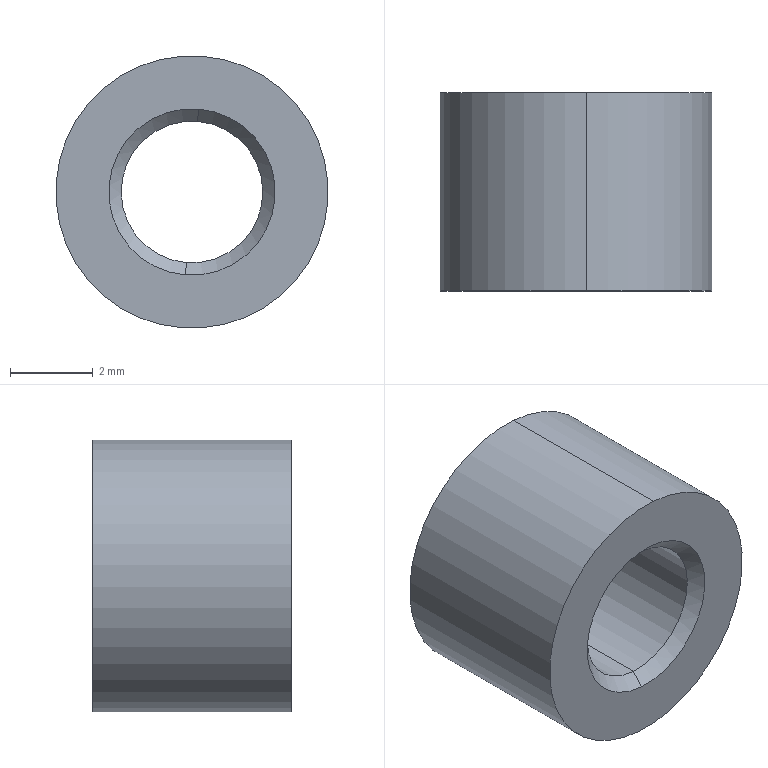Part | STEP file | 2026.6.15-Main Assembly图.sldasm-Part-262 | 1 solid | 10 faces | box 6.6 x 4.8 x 6.6 mm | volume 118.747 mm3 | cylinder 4 | cone 4 | plane 2 | commonest cylinder face diameters 3.433 x2 6.6 x2
STEP:
#1=CARTESIAN_POINT('',(-1616.254,1435.064,3409.798));
#2=VERTEX_POINT('',#1);
#3=CARTESIAN_POINT('',(-1616.254,1439.264,3409.798));
#4=VERTEX_POINT('',#3);
#5=CARTESIAN_POINT('',(-1616.254,1439.564,3409.798));
#6=DIRECTION('',(0.,1.,0.));
#7=VECTOR('',#6,1000.);
#8=LINE('',#5,#7);
#9=EDGE_CURVE('',#2,#4,#8,.T.);
#10=ORIENTED_EDGE('',*,*,#9,.F.);
#11=CARTESIAN_POINT('',(-1616.523,1435.064,3406.375));
#12=VERTEX_POINT('',#11);
#13=CARTESIAN_POINT('',(-1616.388,1435.064,3408.086));
#14=DIRECTION('',(0.,-1.,0.));
#15=DIRECTION('',(0.0785,0.,0.9969));
#16=AXIS2_PLACEMENT_3D('',#13,#14,#15);
#17=CIRCLE('',#16,1.717);
#18=EDGE_CURVE('',#2,#12,#17,.T.);
#19=ORIENTED_EDGE('',*,*,#18,.T.);
#20=CARTESIAN_POINT('',(-1616.523,1439.264,3406.375));
#21=VERTEX_POINT('',#20);
#22=CARTESIAN_POINT('',(-1616.523,1439.564,3406.375));
#23=DIRECTION('',(0.,1.,0.));
#24=VECTOR('',#23,1000.);
#25=LINE('',#22,#24);
#26=EDGE_CURVE('',#12,#21,#25,.T.);
#27=ORIENTED_EDGE('',*,*,#26,.T.);
#28=CARTESIAN_POINT('',(-1616.388,1439.264,3408.086));
#29=DIRECTION('',(0.,1.,0.));
#30=DIRECTION('',(-0.0785,0.,-0.9969));
#31=AXIS2_PLACEMENT_3D('',#28,#29,#30);
#32=CIRCLE('',#31,1.717);
#33=EDGE_CURVE('',#21,#4,#32,.T.);
#34=ORIENTED_EDGE('',*,*,#33,.T.);
#35=EDGE_LOOP('',(#10,#19,#27,#34));
#36=FACE_OUTER_BOUND('',#35,.T.);
#37=CARTESIAN_POINT('',(-1616.388,1439.564,3408.086));
#38=DIRECTION('',(0.,1.,0.));
#39=DIRECTION('',(0.0785,0.,0.9969));
#40=AXIS2_PLACEMENT_3D('',#37,#38,#39);
#41=CYLINDRICAL_SURFACE('',#40,1.717);
#42=ADVANCED_FACE('',(#36),#41,.F.);
#43=CARTESIAN_POINT('',(-1616.547,1434.764,3406.076));
#44=VERTEX_POINT('',#43);
#45=CARTESIAN_POINT('',(-1616.547,1434.764,3406.076));
#46=DIRECTION('',(0.0555,0.7071,0.7049));
#47=VECTOR('',#46,1000.);
#48=LINE('',#45,#47);
#49=EDGE_CURVE('',#44,#12,#48,.T.);
#50=ORIENTED_EDGE('',*,*,#49,.T.);
#51=ORIENTED_EDGE('',*,*,#18,.F.);
#52=CARTESIAN_POINT('',(-1616.23,1434.764,3410.097));
#53=VERTEX_POINT('',#52);
#54=CARTESIAN_POINT('',(-1616.23,1434.764,3410.097));
#55=DIRECTION('',(-0.0555,0.7071,-0.7049));
#56=VECTOR('',#55,1000.);
#57=LINE('',#54,#56);
#58=EDGE_CURVE('',#53,#2,#57,.T.);
#59=ORIENTED_EDGE('',*,*,#58,.F.);
#60=CARTESIAN_POINT('',(-1616.388,1434.764,3408.086));
#61=DIRECTION('',(0.,1.,0.));
#62=DIRECTION('',(0.0785,0.,0.9969));
#63=AXIS2_PLACEMENT_3D('',#60,#61,#62);
#64=CIRCLE('',#63,2.017);
#65=EDGE_CURVE('',#44,#53,#64,.T.);
#66=ORIENTED_EDGE('',*,*,#65,.F.);
#67=EDGE_LOOP('',(#50,#51,#59,#66));
#68=FACE_OUTER_BOUND('',#67,.T.);
#69=CARTESIAN_POINT('',(-1616.388,1434.764,3408.086));
#70=DIRECTION('',(0.,-1.,0.));
#71=DIRECTION('',(-0.0785,0.,-0.9969));
#72=AXIS2_PLACEMENT_3D('',#69,#70,#71);
#73=CONICAL_SURFACE('',#72,2.017,0.7854);
#74=ADVANCED_FACE('',(#68),#73,.F.);
#75=CARTESIAN_POINT('',(-1616.23,1439.564,3410.097));
#76=VERTEX_POINT('',#75);
#77=CARTESIAN_POINT('',(-1616.23,1439.564,3410.097));
#78=DIRECTION('',(0.0555,0.7071,0.7049));
#79=VECTOR('',#78,1000.);
#80=LINE('',#77,#79);
#81=EDGE_CURVE('',#4,#76,#80,.T.);
#82=ORIENTED_EDGE('',*,*,#81,.F.);
#83=ORIENTED_EDGE('',*,*,#33,.F.);
#84=CARTESIAN_POINT('',(-1616.547,1439.564,3406.076));
#85=VERTEX_POINT('',#84);
#86=CARTESIAN_POINT('',(-1616.547,1439.564,3406.076));
#87=DIRECTION('',(-0.0555,0.7071,-0.7049));
#88=VECTOR('',#87,1000.);
#89=LINE('',#86,#88);
#90=EDGE_CURVE('',#21,#85,#89,.T.);
#91=ORIENTED_EDGE('',*,*,#90,.T.);
#92=CARTESIAN_POINT('',(-1616.388,1439.564,3408.086));
#93=DIRECTION('',(0.,1.,0.));
#94=DIRECTION('',(-0.0785,0.,-0.9969));
#95=AXIS2_PLACEMENT_3D('',#92,#93,#94);
#96=CIRCLE('',#95,2.017);
#97=EDGE_CURVE('',#85,#76,#96,.T.);
#98=ORIENTED_EDGE('',*,*,#97,.T.);
#99=EDGE_LOOP('',(#82,#83,#91,#98));
#100=FACE_OUTER_BOUND('',#99,.T.);
#101=CARTESIAN_POINT('',(-1616.388,1439.564,3408.086));
#102=DIRECTION('',(0.,1.,0.));
#103=DIRECTION('',(0.0785,0.,0.9969));
#104=AXIS2_PLACEMENT_3D('',#101,#102,#103);
#105=CONICAL_SURFACE('',#104,2.017,0.7854);
#106=ADVANCED_FACE('',(#100),#105,.F.);
#107=CARTESIAN_POINT('',(-1616.647,1434.764,3404.797));
#108=VERTEX_POINT('',#107);
#109=CARTESIAN_POINT('',(-1616.129,1434.764,3411.376));
#110=VERTEX_POINT('',#109);
#111=CARTESIAN_POINT('',(-1616.388,1434.764,3408.086));
#112=DIRECTION('',(0.,1.,0.));
#113=DIRECTION('',(-0.0785,0.,-0.9969));
#114=AXIS2_PLACEMENT_3D('',#111,#112,#113);
#115=CIRCLE('',#114,3.3);
#116=EDGE_CURVE('',#108,#110,#115,.T.);
#117=ORIENTED_EDGE('',*,*,#116,.F.);
#118=CARTESIAN_POINT('',(-1616.388,1434.764,3408.086));
#119=DIRECTION('',(0.,1.,0.));
#120=DIRECTION('',(-0.0785,0.,-0.9969));
#121=AXIS2_PLACEMENT_3D('',#118,#119,#120);
#122=CIRCLE('',#121,3.3);
#123=EDGE_CURVE('',#110,#108,#122,.T.);
#124=ORIENTED_EDGE('',*,*,#123,.F.);
#125=EDGE_LOOP('',(#117,#124));
#126=FACE_OUTER_BOUND('',#125,.T.);
#127=CARTESIAN_POINT('',(-1616.388,1434.764,3408.086));
#128=DIRECTION('',(0.,1.,0.));
#129=DIRECTION('',(0.0785,0.,0.9969));
#130=AXIS2_PLACEMENT_3D('',#127,#128,#129);
#131=CIRCLE('',#130,2.017);
#132=EDGE_CURVE('',#53,#44,#131,.T.);
#133=ORIENTED_EDGE('',*,*,#132,.T.);
#134=ORIENTED_EDGE('',*,*,#65,.T.);
#135=EDGE_LOOP('',(#133,#134));
#136=FACE_BOUND('',#135,.T.);
#137=CARTESIAN_POINT('',(-1616.388,1434.764,3408.086));
#138=DIRECTION('',(0.,-1.,0.));
#139=DIRECTION('',(0.,0.,-1.));
#140=AXIS2_PLACEMENT_3D('',#137,#138,#139);
#141=PLANE('',#140);
#142=ADVANCED_FACE('',(#126,#136),#141,.T.);
#143=CARTESIAN_POINT('',(-1616.647,1439.564,3404.797));
#144=VERTEX_POINT('',#143);
#145=CARTESIAN_POINT('',(-1616.129,1439.564,3411.376));
#146=VERTEX_POINT('',#145);
#147=CARTESIAN_POINT('',(-1616.388,1439.564,3408.086));
#148=DIRECTION('',(0.,-1.,0.));
#149=DIRECTION('',(-0.0785,0.,-0.9969));
#150=AXIS2_PLACEMENT_3D('',#147,#148,#149);
#151=CIRCLE('',#150,3.3);
#152=EDGE_CURVE('',#144,#146,#151,.T.);
#153=ORIENTED_EDGE('',*,*,#152,.F.);
#154=CARTESIAN_POINT('',(-1616.388,1439.564,3408.086));
#155=DIRECTION('',(0.,-1.,0.));
#156=DIRECTION('',(-0.0785,0.,-0.9969));
#157=AXIS2_PLACEMENT_3D('',#154,#155,#156);
#158=CIRCLE('',#157,3.3);
#159=EDGE_CURVE('',#146,#144,#158,.T.);
#160=ORIENTED_EDGE('',*,*,#159,.F.);
#161=EDGE_LOOP('',(#153,#160));
#162=FACE_OUTER_BOUND('',#161,.T.);
#163=ORIENTED_EDGE('',*,*,#97,.F.);
#164=CARTESIAN_POINT('',(-1616.388,1439.564,3408.086));
#165=DIRECTION('',(0.,1.,0.));
#166=DIRECTION('',(-0.0785,0.,-0.9969));
#167=AXIS2_PLACEMENT_3D('',#164,#165,#166);
#168=CIRCLE('',#167,2.017);
#169=EDGE_CURVE('',#76,#85,#168,.T.);
#170=ORIENTED_EDGE('',*,*,#169,.F.);
#171=EDGE_LOOP('',(#163,#170));
#172=FACE_BOUND('',#171,.T.);
#173=CARTESIAN_POINT('',(-1616.388,1439.564,3408.086));
#174=DIRECTION('',(0.,-1.,0.));
#175=DIRECTION('',(0.,0.,-1.));
#176=AXIS2_PLACEMENT_3D('',#173,#174,#175);
#177=PLANE('',#176);
#178=ADVANCED_FACE('',(#162,#172),#177,.F.);
#179=CARTESIAN_POINT('',(-1616.129,1439.564,3411.376));
#180=DIRECTION('',(0.,1.,0.));
#181=VECTOR('',#180,1000.);
#182=LINE('',#179,#181);
#183=EDGE_CURVE('',#110,#146,#182,.T.);
#184=ORIENTED_EDGE('',*,*,#183,.F.);
#185=ORIENTED_EDGE('',*,*,#123,.T.);
#186=CARTESIAN_POINT('',(-1616.647,1439.564,3404.797));
#187=DIRECTION('',(0.,1.,0.));
#188=VECTOR('',#187,1000.);
#189=LINE('',#186,#188);
#190=EDGE_CURVE('',#108,#144,#189,.T.);
#191=ORIENTED_EDGE('',*,*,#190,.T.);
#192=ORIENTED_EDGE('',*,*,#152,.T.);
#193=EDGE_LOOP('',(#184,#185,#191,#192));
#194=FACE_OUTER_BOUND('',#193,.T.);
#195=CARTESIAN_POINT('',(-1616.388,1439.564,3408.086));
#196=DIRECTION('',(0.,1.,0.));
#197=DIRECTION('',(0.0785,0.,0.9969));
#198=AXIS2_PLACEMENT_3D('',#195,#196,#197);
#199=CYLINDRICAL_SURFACE('',#198,3.3);
#200=ADVANCED_FACE('',(#194),#199,.T.);
#201=CARTESIAN_POINT('',(-1616.388,1435.064,3408.086));
#202=DIRECTION('',(0.,-1.,0.));
#203=DIRECTION('',(0.0785,0.,0.9969));
#204=AXIS2_PLACEMENT_3D('',#201,#202,#203);
#205=CIRCLE('',#204,1.717);
#206=EDGE_CURVE('',#12,#2,#205,.T.);
#207=ORIENTED_EDGE('',*,*,#206,.T.);
#208=ORIENTED_EDGE('',*,*,#9,.T.);
#209=CARTESIAN_POINT('',(-1616.388,1439.264,3408.086));
#210=DIRECTION('',(0.,1.,0.));
#211=DIRECTION('',(-0.0785,0.,-0.9969));
#212=AXIS2_PLACEMENT_3D('',#209,#210,#211);
#213=CIRCLE('',#212,1.717);
#214=EDGE_CURVE('',#4,#21,#213,.T.);
#215=ORIENTED_EDGE('',*,*,#214,.T.);
#216=ORIENTED_EDGE('',*,*,#26,.F.);
#217=EDGE_LOOP('',(#207,#208,#215,#216));
#218=FACE_OUTER_BOUND('',#217,.T.);
#219=CARTESIAN_POINT('',(-1616.388,1439.564,3408.086));
#220=DIRECTION('',(0.,1.,0.));
#221=DIRECTION('',(0.0785,0.,0.9969));
#222=AXIS2_PLACEMENT_3D('',#219,#220,#221);
#223=CYLINDRICAL_SURFACE('',#222,1.717);
#224=ADVANCED_FACE('',(#218),#223,.F.);
#225=ORIENTED_EDGE('',*,*,#206,.F.);
#226=ORIENTED_EDGE('',*,*,#49,.F.);
#227=ORIENTED_EDGE('',*,*,#132,.F.);
#228=ORIENTED_EDGE('',*,*,#58,.T.);
#229=EDGE_LOOP('',(#225,#226,#227,#228));
#230=FACE_OUTER_BOUND('',#229,.T.);
#231=CARTESIAN_POINT('',(-1616.388,1434.764,3408.086));
#232=DIRECTION('',(0.,-1.,0.));
#233=DIRECTION('',(-0.0785,0.,-0.9969));
#234=AXIS2_PLACEMENT_3D('',#231,#232,#233);
#235=CONICAL_SURFACE('',#234,2.017,0.7854);
#236=ADVANCED_FACE('',(#230),#235,.F.);
#237=ORIENTED_EDGE('',*,*,#214,.F.);
#238=ORIENTED_EDGE('',*,*,#81,.T.);
#239=ORIENTED_EDGE('',*,*,#169,.T.);
#240=ORIENTED_EDGE('',*,*,#90,.F.);
#241=EDGE_LOOP('',(#237,#238,#239,#240));
#242=FACE_OUTER_BOUND('',#241,.T.);
#243=CARTESIAN_POINT('',(-1616.388,1439.564,3408.086));
#244=DIRECTION('',(0.,1.,0.));
#245=DIRECTION('',(0.0785,0.,0.9969));
#246=AXIS2_PLACEMENT_3D('',#243,#244,#245);
#247=CONICAL_SURFACE('',#246,2.017,0.7854);
#248=ADVANCED_FACE('',(#242),#247,.F.);
#249=ORIENTED_EDGE('',*,*,#116,.T.);
#250=ORIENTED_EDGE('',*,*,#183,.T.);
#251=ORIENTED_EDGE('',*,*,#159,.T.);
#252=ORIENTED_EDGE('',*,*,#190,.F.);
#253=EDGE_LOOP('',(#249,#250,#251,#252));
#254=FACE_OUTER_BOUND('',#253,.T.);
#255=CARTESIAN_POINT('',(-1616.388,1439.564,3408.086));
#256=DIRECTION('',(0.,1.,0.));
#257=DIRECTION('',(0.0785,0.,0.9969));
#258=AXIS2_PLACEMENT_3D('',#255,#256,#257);
#259=CYLINDRICAL_SURFACE('',#258,3.3);
#260=ADVANCED_FACE('',(#254),#259,.T.);
#261=CLOSED_SHELL('',(#42,#74,#106,#142,#178,#200,#224,#236,#248,#260));
#262=MANIFOLD_SOLID_BREP('',#261);
#263=CARTESIAN_POINT('',(0.,0.,0.));
#264=DIRECTION('',(0.,0.,1.));
#265=DIRECTION('',(1.,0.,0.));
#266=AXIS2_PLACEMENT_3D('',#263,#264,#265);
#267=(LENGTH_UNIT()NAMED_UNIT(*)SI_UNIT(.MILLI.,.METRE.));
#268=UNCERTAINTY_MEASURE_WITH_UNIT(LENGTH_MEASURE(0.00001),#267,'','');
#269=(NAMED_UNIT(*)PLANE_ANGLE_UNIT()SI_UNIT($,.RADIAN.));
#270=(NAMED_UNIT(*)SI_UNIT($,.STERADIAN.)SOLID_ANGLE_UNIT());
#271=(GEOMETRIC_REPRESENTATION_CONTEXT(3)GLOBAL_UNCERTAINTY_ASSIGNED_CONTEXT((#268))GLOBAL_UNIT_ASSIGNED_CONTEXT((#267,#269,#270))REPRESENTATION_CONTEXT('',''));
#272=ADVANCED_BREP_SHAPE_REPRESENTATION('',(#262,#266),#271);